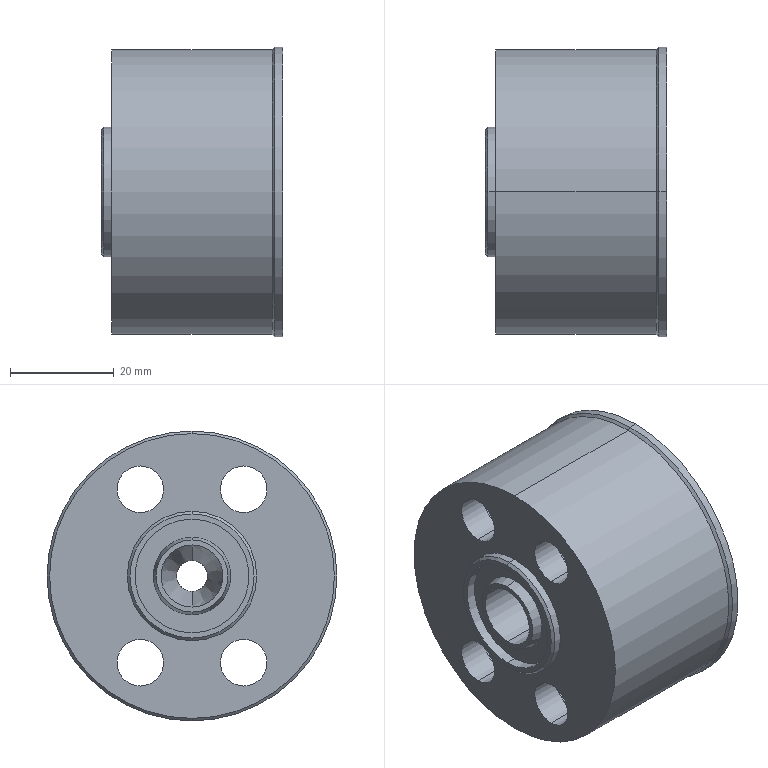Part | STEP file | NL23,33(NL23_SR21(D4-D8)) | 1 solid | 57 faces | box 35 x 56 x 56 mm | volume 57560 mm3 | cylinder 28 | cone 16 | plane 9 | sphere 4 | commonest cylinder face diameters 9 x8 14 x8 6 x2 12 x2 22 x2 25 x2